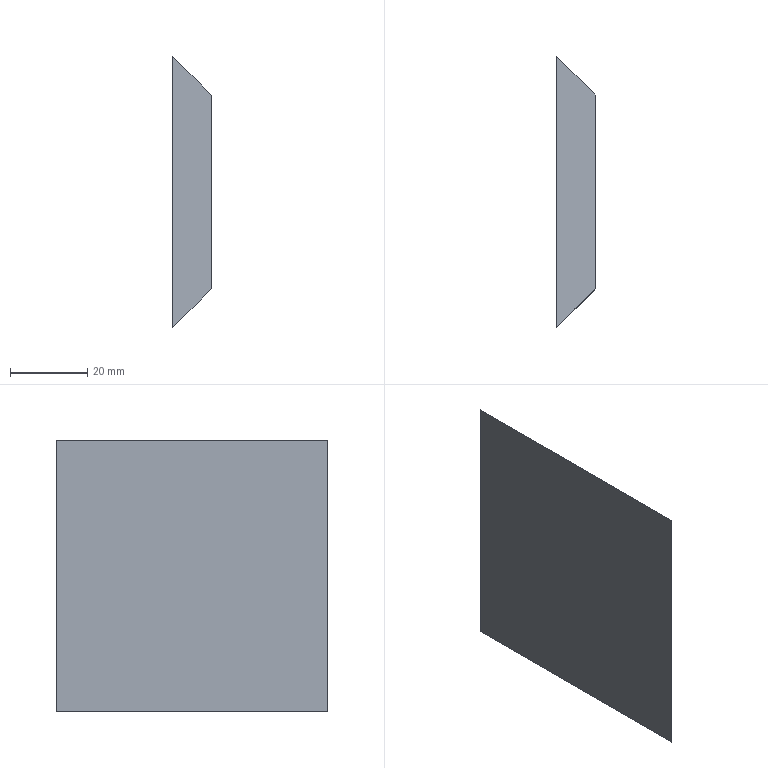Part | NX | features solid 2 | 1 solid | 6 faces | box 10 x 70 x 70 mm | volume 36333 mm3 | plane 6
STEP:
#1=CARTESIAN_POINT('',(1445.,530.,25.));
#2=VERTEX_POINT('',#1);
#3=CARTESIAN_POINT('',(1445.,480.,25.));
#4=VERTEX_POINT('',#3);
#5=CARTESIAN_POINT('',(1445.,470.,25.));
#6=DIRECTION('',(0.,-1.,0.));
#7=VECTOR('',#6,1000.);
#8=LINE('',#5,#7);
#9=EDGE_CURVE('',#2,#4,#8,.T.);
#10=ORIENTED_EDGE('',*,*,#9,.T.);
#11=CARTESIAN_POINT('',(1445.,480.,-25.));
#12=VERTEX_POINT('',#11);
#13=CARTESIAN_POINT('',(1445.,480.,-35.));
#14=DIRECTION('',(0.,0.,-1.));
#15=VECTOR('',#14,1000.);
#16=LINE('',#13,#15);
#17=EDGE_CURVE('',#4,#12,#16,.T.);
#18=ORIENTED_EDGE('',*,*,#17,.T.);
#19=CARTESIAN_POINT('',(1445.,530.,-25.));
#20=VERTEX_POINT('',#19);
#21=CARTESIAN_POINT('',(1445.,470.,-25.));
#22=DIRECTION('',(0.,1.,0.));
#23=VECTOR('',#22,1000.);
#24=LINE('',#21,#23);
#25=EDGE_CURVE('',#12,#20,#24,.T.);
#26=ORIENTED_EDGE('',*,*,#25,.T.);
#27=CARTESIAN_POINT('',(1445.,530.,-35.));
#28=DIRECTION('',(0.,0.,1.));
#29=VECTOR('',#28,1000.);
#30=LINE('',#27,#29);
#31=EDGE_CURVE('',#20,#2,#30,.T.);
#32=ORIENTED_EDGE('',*,*,#31,.T.);
#33=EDGE_LOOP('',(#10,#18,#26,#32));
#34=FACE_BOUND('',#33,.T.);
#35=CARTESIAN_POINT('',(1445.,470.,-35.));
#36=DIRECTION('',(1.,0.,0.));
#37=DIRECTION('',(0.,0.,-1.));
#38=AXIS2_PLACEMENT_3D('',#35,#36,#37);
#39=PLANE('',#38);
#40=ADVANCED_FACE('',(#34),#39,.T.);
#41=CARTESIAN_POINT('',(1435.,470.,35.));
#42=VERTEX_POINT('',#41);
#43=CARTESIAN_POINT('',(1435.,540.,35.));
#44=VERTEX_POINT('',#43);
#45=CARTESIAN_POINT('',(1435.,470.,35.));
#46=DIRECTION('',(0.,1.,0.));
#47=VECTOR('',#46,1000.);
#48=LINE('',#45,#47);
#49=EDGE_CURVE('',#42,#44,#48,.T.);
#50=ORIENTED_EDGE('',*,*,#49,.T.);
#51=CARTESIAN_POINT('',(1435.,540.,-35.));
#52=VERTEX_POINT('',#51);
#53=CARTESIAN_POINT('',(1435.,540.,-35.));
#54=DIRECTION('',(0.,0.,1.));
#55=VECTOR('',#54,1000.);
#56=LINE('',#53,#55);
#57=EDGE_CURVE('',#52,#44,#56,.T.);
#58=ORIENTED_EDGE('',*,*,#57,.F.);
#59=CARTESIAN_POINT('',(1435.,470.,-35.));
#60=VERTEX_POINT('',#59);
#61=CARTESIAN_POINT('',(1435.,470.,-35.));
#62=DIRECTION('',(0.,1.,0.));
#63=VECTOR('',#62,1000.);
#64=LINE('',#61,#63);
#65=EDGE_CURVE('',#60,#52,#64,.T.);
#66=ORIENTED_EDGE('',*,*,#65,.F.);
#67=CARTESIAN_POINT('',(1435.,470.,-35.));
#68=DIRECTION('',(0.,0.,1.));
#69=VECTOR('',#68,1000.);
#70=LINE('',#67,#69);
#71=EDGE_CURVE('',#60,#42,#70,.T.);
#72=ORIENTED_EDGE('',*,*,#71,.T.);
#73=EDGE_LOOP('',(#50,#58,#66,#72));
#74=FACE_BOUND('',#73,.T.);
#75=CARTESIAN_POINT('',(1435.,470.,-35.));
#76=DIRECTION('',(1.,0.,0.));
#77=DIRECTION('',(0.,0.,-1.));
#78=AXIS2_PLACEMENT_3D('',#75,#76,#77);
#79=PLANE('',#78);
#80=ADVANCED_FACE('',(#74),#79,.F.);
#81=CARTESIAN_POINT('',(1465.,510.,5.));
#82=DIRECTION('',(-0.5774,0.5774,0.5774));
#83=VECTOR('',#82,1000.);
#84=LINE('',#81,#83);
#85=EDGE_CURVE('',#2,#44,#84,.T.);
#86=ORIENTED_EDGE('',*,*,#85,.F.);
#87=ORIENTED_EDGE('',*,*,#31,.F.);
#88=CARTESIAN_POINT('',(1465.,510.,-5.));
#89=DIRECTION('',(0.5774,-0.5774,0.5774));
#90=VECTOR('',#89,1000.);
#91=LINE('',#88,#90);
#92=EDGE_CURVE('',#52,#20,#91,.T.);
#93=ORIENTED_EDGE('',*,*,#92,.F.);
#94=ORIENTED_EDGE('',*,*,#57,.T.);
#95=EDGE_LOOP('',(#86,#87,#93,#94));
#96=FACE_BOUND('',#95,.T.);
#97=CARTESIAN_POINT('',(1445.,530.,-35.));
#98=DIRECTION('',(-0.7071,-0.7071,0.));
#99=DIRECTION('',(0.7071,-0.7071,0.));
#100=AXIS2_PLACEMENT_3D('',#97,#98,#99);
#101=PLANE('',#100);
#102=ADVANCED_FACE('',(#96),#101,.F.);
#103=ORIENTED_EDGE('',*,*,#92,.T.);
#104=ORIENTED_EDGE('',*,*,#25,.F.);
#105=CARTESIAN_POINT('',(1441.667,476.667,-28.333));
#106=DIRECTION('',(0.5774,0.5774,0.5774));
#107=VECTOR('',#106,1000.);
#108=LINE('',#105,#107);
#109=EDGE_CURVE('',#60,#12,#108,.T.);
#110=ORIENTED_EDGE('',*,*,#109,.F.);
#111=ORIENTED_EDGE('',*,*,#65,.T.);
#112=EDGE_LOOP('',(#103,#104,#110,#111));
#113=FACE_BOUND('',#112,.T.);
#114=CARTESIAN_POINT('',(1445.,470.,-25.));
#115=DIRECTION('',(-0.7071,0.,0.7071));
#116=DIRECTION('',(0.7071,0.,0.7071));
#117=AXIS2_PLACEMENT_3D('',#114,#115,#116);
#118=PLANE('',#117);
#119=ADVANCED_FACE('',(#113),#118,.F.);
#120=ORIENTED_EDGE('',*,*,#85,.T.);
#121=ORIENTED_EDGE('',*,*,#49,.F.);
#122=CARTESIAN_POINT('',(1435.,470.,35.));
#123=DIRECTION('',(0.5774,0.5774,-0.5774));
#124=VECTOR('',#123,1000.);
#125=LINE('',#122,#124);
#126=EDGE_CURVE('',#4,#42,#125,.F.);
#127=ORIENTED_EDGE('',*,*,#126,.F.);
#128=ORIENTED_EDGE('',*,*,#9,.F.);
#129=EDGE_LOOP('',(#120,#121,#127,#128));
#130=FACE_BOUND('',#129,.T.);
#131=CARTESIAN_POINT('',(1435.,470.,35.));
#132=DIRECTION('',(0.7071,0.,0.7071));
#133=DIRECTION('',(0.7071,0.,-0.7071));
#134=AXIS2_PLACEMENT_3D('',#131,#132,#133);
#135=PLANE('',#134);
#136=ADVANCED_FACE('',(#130),#135,.T.);
#137=ORIENTED_EDGE('',*,*,#109,.T.);
#138=ORIENTED_EDGE('',*,*,#17,.F.);
#139=ORIENTED_EDGE('',*,*,#126,.T.);
#140=ORIENTED_EDGE('',*,*,#71,.F.);
#141=EDGE_LOOP('',(#137,#138,#139,#140));
#142=FACE_BOUND('',#141,.T.);
#143=CARTESIAN_POINT('',(1435.,470.,-35.));
#144=DIRECTION('',(0.7071,-0.7071,0.));
#145=DIRECTION('',(0.7071,0.7071,0.));
#146=AXIS2_PLACEMENT_3D('',#143,#144,#145);
#147=PLANE('',#146);
#148=ADVANCED_FACE('',(#142),#147,.T.);
#149=CLOSED_SHELL('',(#40,#80,#102,#119,#136,#148));
#150=MANIFOLD_SOLID_BREP('',#149);
#151=(LENGTH_UNIT()NAMED_UNIT(*)SI_UNIT(.MILLI.,.METRE.));
#152=UNCERTAINTY_MEASURE_WITH_UNIT(LENGTH_MEASURE(0.00001),#151,'','');
#153=(NAMED_UNIT(*)PLANE_ANGLE_UNIT()SI_UNIT($,.RADIAN.));
#154=(NAMED_UNIT(*)SI_UNIT($,.STERADIAN.)SOLID_ANGLE_UNIT());
#155=(GEOMETRIC_REPRESENTATION_CONTEXT(3)GLOBAL_UNCERTAINTY_ASSIGNED_CONTEXT((#152))GLOBAL_UNIT_ASSIGNED_CONTEXT((#151,#153,#154))REPRESENTATION_CONTEXT('',''));
#156=ADVANCED_BREP_SHAPE_REPRESENTATION('',(#150),#155);